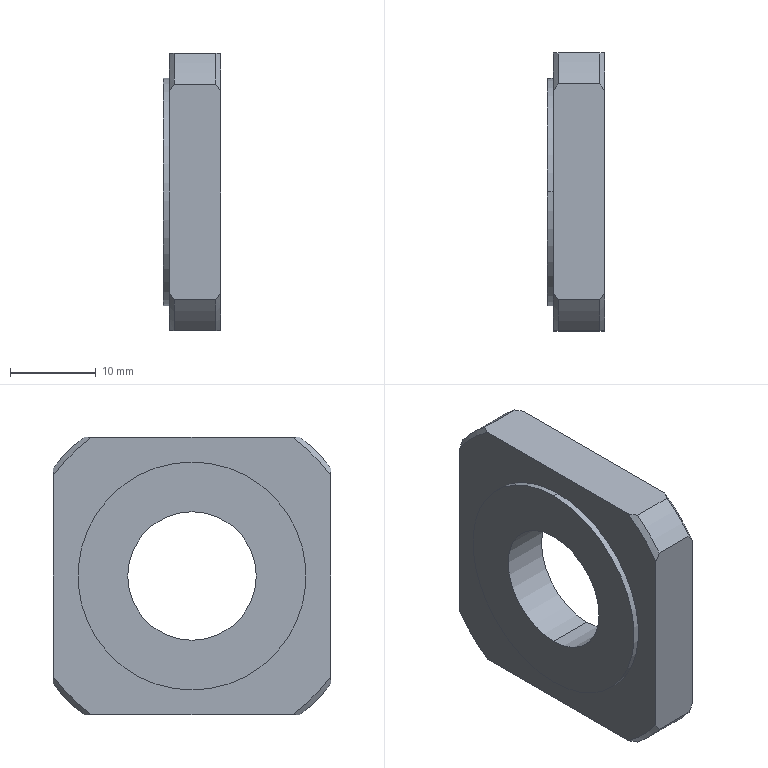Part | STEP file | 12bswcov | 1 solid | 86 faces | box 6.7 x 32.4 x 32.4 mm | volume 4942 mm3 | plane 44 | cylinder 26 | torus 8 | cone 8 | commonest cylinder face diameters 5.04 x8 5.64 x8 41.04 x4 15 x2 22.8 x2 26.6 x2